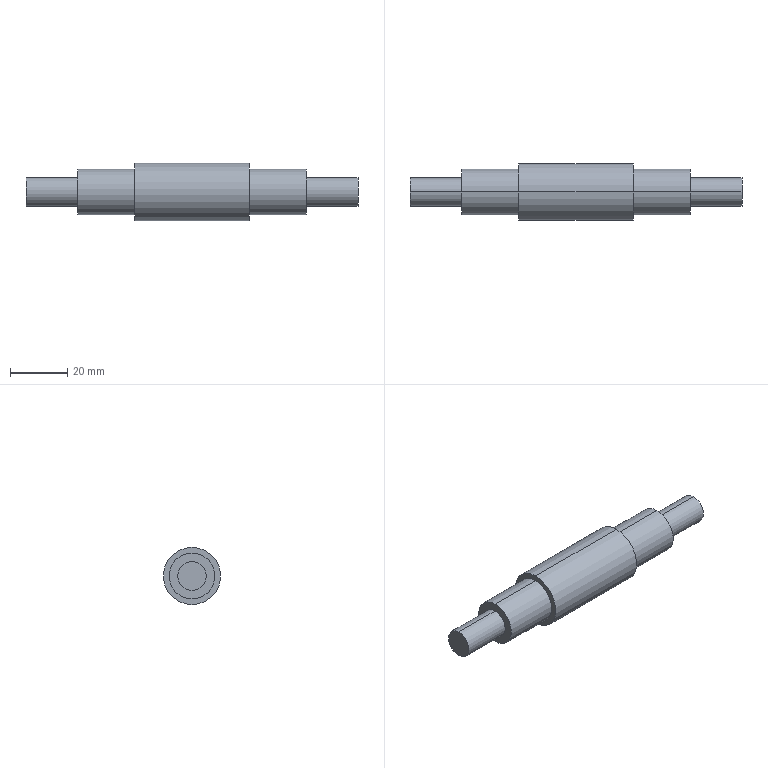Part | SolidWorks | features BaseBody 1 | 1 solid | 16 faces | box 116 x 20 x 20 mm | volume 23436 mm3 | cylinder 10 | plane 6 | commonest cylinder face diameters 10 x4 16 x4 20 x2
STEP:
#1=CARTESIAN_POINT('',(78.,0.,-5.));
#2=VERTEX_POINT('',#1);
#3=CARTESIAN_POINT('',(78.,0.,5.));
#4=VERTEX_POINT('',#3);
#5=CARTESIAN_POINT('',(78.,0.,0.));
#6=DIRECTION('',(1.,0.,0.));
#7=DIRECTION('',(0.,0.,-1.));
#8=AXIS2_PLACEMENT_3D('',#5,#6,#7);
#9=CIRCLE('',#8,5.);
#10=EDGE_CURVE('',#2,#4,#9,.T.);
#11=ORIENTED_EDGE('',*,*,#10,.F.);
#12=CARTESIAN_POINT('',(60.,0.,-5.));
#13=VERTEX_POINT('',#12);
#14=CARTESIAN_POINT('',(78.,0.,-5.));
#15=DIRECTION('',(-1.,0.,0.));
#16=VECTOR('',#15,1000.);
#17=LINE('',#14,#16);
#18=EDGE_CURVE('',#2,#13,#17,.T.);
#19=ORIENTED_EDGE('',*,*,#18,.T.);
#20=CARTESIAN_POINT('',(60.,0.,5.));
#21=VERTEX_POINT('',#20);
#22=CARTESIAN_POINT('',(60.,0.,0.));
#23=DIRECTION('',(1.,0.,0.));
#24=DIRECTION('',(0.,0.,-1.));
#25=AXIS2_PLACEMENT_3D('',#22,#23,#24);
#26=CIRCLE('',#25,5.);
#27=EDGE_CURVE('',#13,#21,#26,.T.);
#28=ORIENTED_EDGE('',*,*,#27,.T.);
#29=CARTESIAN_POINT('',(78.,0.,5.));
#30=DIRECTION('',(-1.,0.,0.));
#31=VECTOR('',#30,1000.);
#32=LINE('',#29,#31);
#33=EDGE_CURVE('',#4,#21,#32,.T.);
#34=ORIENTED_EDGE('',*,*,#33,.F.);
#35=EDGE_LOOP('',(#11,#19,#28,#34));
#36=FACE_OUTER_BOUND('',#35,.T.);
#37=CARTESIAN_POINT('',(78.,0.,0.));
#38=DIRECTION('',(-1.,0.,0.));
#39=DIRECTION('',(0.,0.,1.));
#40=AXIS2_PLACEMENT_3D('',#37,#38,#39);
#41=CYLINDRICAL_SURFACE('',#40,5.);
#42=ADVANCED_FACE('',(#36),#41,.T.);
#43=CARTESIAN_POINT('',(-38.,0.,5.));
#44=VERTEX_POINT('',#43);
#45=CARTESIAN_POINT('',(-38.,0.,-5.));
#46=VERTEX_POINT('',#45);
#47=CARTESIAN_POINT('',(-38.,0.,0.));
#48=DIRECTION('',(-1.,0.,0.));
#49=DIRECTION('',(0.,0.,1.));
#50=AXIS2_PLACEMENT_3D('',#47,#48,#49);
#51=CIRCLE('',#50,5.);
#52=EDGE_CURVE('',#44,#46,#51,.T.);
#53=ORIENTED_EDGE('',*,*,#52,.F.);
#54=CARTESIAN_POINT('',(-20.,0.,5.));
#55=VERTEX_POINT('',#54);
#56=CARTESIAN_POINT('',(-38.,0.,5.));
#57=DIRECTION('',(1.,0.,0.));
#58=VECTOR('',#57,1000.);
#59=LINE('',#56,#58);
#60=EDGE_CURVE('',#44,#55,#59,.T.);
#61=ORIENTED_EDGE('',*,*,#60,.T.);
#62=CARTESIAN_POINT('',(-20.,0.,-5.));
#63=VERTEX_POINT('',#62);
#64=CARTESIAN_POINT('',(-20.,0.,0.));
#65=DIRECTION('',(-1.,0.,0.));
#66=DIRECTION('',(0.,0.,1.));
#67=AXIS2_PLACEMENT_3D('',#64,#65,#66);
#68=CIRCLE('',#67,5.);
#69=EDGE_CURVE('',#55,#63,#68,.T.);
#70=ORIENTED_EDGE('',*,*,#69,.T.);
#71=CARTESIAN_POINT('',(-38.,0.,-5.));
#72=DIRECTION('',(1.,0.,0.));
#73=VECTOR('',#72,1000.);
#74=LINE('',#71,#73);
#75=EDGE_CURVE('',#46,#63,#74,.T.);
#76=ORIENTED_EDGE('',*,*,#75,.F.);
#77=EDGE_LOOP('',(#53,#61,#70,#76));
#78=FACE_OUTER_BOUND('',#77,.T.);
#79=CARTESIAN_POINT('',(-38.,0.,0.));
#80=DIRECTION('',(1.,0.,0.));
#81=DIRECTION('',(0.,0.,-1.));
#82=AXIS2_PLACEMENT_3D('',#79,#80,#81);
#83=CYLINDRICAL_SURFACE('',#82,5.);
#84=ADVANCED_FACE('',(#78),#83,.T.);
#85=CARTESIAN_POINT('',(-20.,0.,8.));
#86=VERTEX_POINT('',#85);
#87=CARTESIAN_POINT('',(-20.,0.,-8.));
#88=VERTEX_POINT('',#87);
#89=CARTESIAN_POINT('',(-20.,0.,0.));
#90=DIRECTION('',(-1.,0.,0.));
#91=DIRECTION('',(0.,0.,1.));
#92=AXIS2_PLACEMENT_3D('',#89,#90,#91);
#93=CIRCLE('',#92,8.);
#94=EDGE_CURVE('',#86,#88,#93,.T.);
#95=ORIENTED_EDGE('',*,*,#94,.F.);
#96=CARTESIAN_POINT('',(0.,0.,8.));
#97=VERTEX_POINT('',#96);
#98=CARTESIAN_POINT('',(-20.,0.,8.));
#99=DIRECTION('',(1.,0.,0.));
#100=VECTOR('',#99,1000.);
#101=LINE('',#98,#100);
#102=EDGE_CURVE('',#86,#97,#101,.T.);
#103=ORIENTED_EDGE('',*,*,#102,.T.);
#104=CARTESIAN_POINT('',(0.,0.,-8.));
#105=VERTEX_POINT('',#104);
#106=CARTESIAN_POINT('',(0.,0.,0.));
#107=DIRECTION('',(-1.,0.,0.));
#108=DIRECTION('',(0.,0.,1.));
#109=AXIS2_PLACEMENT_3D('',#106,#107,#108);
#110=CIRCLE('',#109,8.);
#111=EDGE_CURVE('',#97,#105,#110,.T.);
#112=ORIENTED_EDGE('',*,*,#111,.T.);
#113=CARTESIAN_POINT('',(-20.,0.,-8.));
#114=DIRECTION('',(1.,0.,0.));
#115=VECTOR('',#114,1000.);
#116=LINE('',#113,#115);
#117=EDGE_CURVE('',#88,#105,#116,.T.);
#118=ORIENTED_EDGE('',*,*,#117,.F.);
#119=EDGE_LOOP('',(#95,#103,#112,#118));
#120=FACE_OUTER_BOUND('',#119,.T.);
#121=CARTESIAN_POINT('',(-20.,0.,0.));
#122=DIRECTION('',(1.,0.,0.));
#123=DIRECTION('',(0.,0.,-1.));
#124=AXIS2_PLACEMENT_3D('',#121,#122,#123);
#125=CYLINDRICAL_SURFACE('',#124,8.);
#126=ADVANCED_FACE('',(#120),#125,.T.);
#127=CARTESIAN_POINT('',(60.,0.,-8.));
#128=VERTEX_POINT('',#127);
#129=CARTESIAN_POINT('',(60.,0.,8.));
#130=VERTEX_POINT('',#129);
#131=CARTESIAN_POINT('',(60.,0.,0.));
#132=DIRECTION('',(1.,0.,0.));
#133=DIRECTION('',(0.,0.,-1.));
#134=AXIS2_PLACEMENT_3D('',#131,#132,#133);
#135=CIRCLE('',#134,8.);
#136=EDGE_CURVE('',#128,#130,#135,.T.);
#137=ORIENTED_EDGE('',*,*,#136,.F.);
#138=CARTESIAN_POINT('',(40.,0.,-8.));
#139=VERTEX_POINT('',#138);
#140=CARTESIAN_POINT('',(60.,0.,-8.));
#141=DIRECTION('',(-1.,0.,0.));
#142=VECTOR('',#141,1000.);
#143=LINE('',#140,#142);
#144=EDGE_CURVE('',#128,#139,#143,.T.);
#145=ORIENTED_EDGE('',*,*,#144,.T.);
#146=CARTESIAN_POINT('',(40.,0.,8.));
#147=VERTEX_POINT('',#146);
#148=CARTESIAN_POINT('',(40.,0.,0.));
#149=DIRECTION('',(1.,0.,0.));
#150=DIRECTION('',(0.,0.,-1.));
#151=AXIS2_PLACEMENT_3D('',#148,#149,#150);
#152=CIRCLE('',#151,8.);
#153=EDGE_CURVE('',#139,#147,#152,.T.);
#154=ORIENTED_EDGE('',*,*,#153,.T.);
#155=CARTESIAN_POINT('',(60.,0.,8.));
#156=DIRECTION('',(-1.,0.,0.));
#157=VECTOR('',#156,1000.);
#158=LINE('',#155,#157);
#159=EDGE_CURVE('',#130,#147,#158,.T.);
#160=ORIENTED_EDGE('',*,*,#159,.F.);
#161=EDGE_LOOP('',(#137,#145,#154,#160));
#162=FACE_OUTER_BOUND('',#161,.T.);
#163=CARTESIAN_POINT('',(60.,0.,0.));
#164=DIRECTION('',(-1.,0.,0.));
#165=DIRECTION('',(0.,0.,1.));
#166=AXIS2_PLACEMENT_3D('',#163,#164,#165);
#167=CYLINDRICAL_SURFACE('',#166,8.);
#168=ADVANCED_FACE('',(#162),#167,.T.);
#169=CARTESIAN_POINT('',(40.,0.,-10.));
#170=VERTEX_POINT('',#169);
#171=CARTESIAN_POINT('',(40.,0.,10.));
#172=VERTEX_POINT('',#171);
#173=CARTESIAN_POINT('',(40.,0.,0.));
#174=DIRECTION('',(1.,0.,0.));
#175=DIRECTION('',(0.,0.,-1.));
#176=AXIS2_PLACEMENT_3D('',#173,#174,#175);
#177=CIRCLE('',#176,10.);
#178=EDGE_CURVE('',#170,#172,#177,.T.);
#179=ORIENTED_EDGE('',*,*,#178,.F.);
#180=CARTESIAN_POINT('',(0.,0.,-10.));
#181=VERTEX_POINT('',#180);
#182=CARTESIAN_POINT('',(40.,0.,-10.));
#183=DIRECTION('',(-1.,0.,0.));
#184=VECTOR('',#183,1000.);
#185=LINE('',#182,#184);
#186=EDGE_CURVE('',#170,#181,#185,.T.);
#187=ORIENTED_EDGE('',*,*,#186,.T.);
#188=CARTESIAN_POINT('',(0.,0.,10.));
#189=VERTEX_POINT('',#188);
#190=CARTESIAN_POINT('',(0.,0.,0.));
#191=DIRECTION('',(1.,0.,0.));
#192=DIRECTION('',(0.,0.,-1.));
#193=AXIS2_PLACEMENT_3D('',#190,#191,#192);
#194=CIRCLE('',#193,10.);
#195=EDGE_CURVE('',#181,#189,#194,.T.);
#196=ORIENTED_EDGE('',*,*,#195,.T.);
#197=CARTESIAN_POINT('',(40.,0.,10.));
#198=DIRECTION('',(-1.,0.,0.));
#199=VECTOR('',#198,1000.);
#200=LINE('',#197,#199);
#201=EDGE_CURVE('',#172,#189,#200,.T.);
#202=ORIENTED_EDGE('',*,*,#201,.F.);
#203=EDGE_LOOP('',(#179,#187,#196,#202));
#204=FACE_OUTER_BOUND('',#203,.T.);
#205=CARTESIAN_POINT('',(40.,0.,0.));
#206=DIRECTION('',(-1.,0.,0.));
#207=DIRECTION('',(0.,0.,1.));
#208=AXIS2_PLACEMENT_3D('',#205,#206,#207);
#209=CYLINDRICAL_SURFACE('',#208,10.);
#210=ADVANCED_FACE('',(#204),#209,.T.);
#211=ORIENTED_EDGE('',*,*,#186,.F.);
#212=CARTESIAN_POINT('',(40.,0.,0.));
#213=DIRECTION('',(1.,0.,0.));
#214=DIRECTION('',(0.,0.,-1.));
#215=AXIS2_PLACEMENT_3D('',#212,#213,#214);
#216=CIRCLE('',#215,10.);
#217=EDGE_CURVE('',#172,#170,#216,.T.);
#218=ORIENTED_EDGE('',*,*,#217,.F.);
#219=ORIENTED_EDGE('',*,*,#201,.T.);
#220=CARTESIAN_POINT('',(0.,0.,0.));
#221=DIRECTION('',(1.,0.,0.));
#222=DIRECTION('',(0.,0.,-1.));
#223=AXIS2_PLACEMENT_3D('',#220,#221,#222);
#224=CIRCLE('',#223,10.);
#225=EDGE_CURVE('',#189,#181,#224,.T.);
#226=ORIENTED_EDGE('',*,*,#225,.T.);
#227=EDGE_LOOP('',(#211,#218,#219,#226));
#228=FACE_OUTER_BOUND('',#227,.T.);
#229=CARTESIAN_POINT('',(40.,0.,0.));
#230=DIRECTION('',(-1.,0.,0.));
#231=DIRECTION('',(0.,0.,1.));
#232=AXIS2_PLACEMENT_3D('',#229,#230,#231);
#233=CYLINDRICAL_SURFACE('',#232,10.);
#234=ADVANCED_FACE('',(#228),#233,.T.);
#235=CARTESIAN_POINT('',(40.,0.,0.));
#236=DIRECTION('',(1.,0.,0.));
#237=DIRECTION('',(0.,0.,-1.));
#238=AXIS2_PLACEMENT_3D('',#235,#236,#237);
#239=CIRCLE('',#238,8.);
#240=EDGE_CURVE('',#147,#139,#239,.T.);
#241=ORIENTED_EDGE('',*,*,#240,.F.);
#242=ORIENTED_EDGE('',*,*,#153,.F.);
#243=EDGE_LOOP('',(#241,#242));
#244=FACE_BOUND('',#243,.T.);
#245=ORIENTED_EDGE('',*,*,#217,.T.);
#246=ORIENTED_EDGE('',*,*,#178,.T.);
#247=EDGE_LOOP('',(#245,#246));
#248=FACE_OUTER_BOUND('',#247,.T.);
#249=CARTESIAN_POINT('',(40.,0.,0.));
#250=DIRECTION('',(1.,0.,0.));
#251=DIRECTION('',(0.,0.,-1.));
#252=AXIS2_PLACEMENT_3D('',#249,#250,#251);
#253=PLANE('',#252);
#254=ADVANCED_FACE('',(#244,#248),#253,.T.);
#255=CARTESIAN_POINT('',(0.,0.,0.));
#256=DIRECTION('',(-1.,0.,0.));
#257=DIRECTION('',(0.,0.,1.));
#258=AXIS2_PLACEMENT_3D('',#255,#256,#257);
#259=CIRCLE('',#258,8.);
#260=EDGE_CURVE('',#105,#97,#259,.T.);
#261=ORIENTED_EDGE('',*,*,#260,.F.);
#262=ORIENTED_EDGE('',*,*,#111,.F.);
#263=EDGE_LOOP('',(#261,#262));
#264=FACE_BOUND('',#263,.T.);
#265=ORIENTED_EDGE('',*,*,#225,.F.);
#266=ORIENTED_EDGE('',*,*,#195,.F.);
#267=EDGE_LOOP('',(#265,#266));
#268=FACE_OUTER_BOUND('',#267,.T.);
#269=CARTESIAN_POINT('',(0.,0.,0.));
#270=DIRECTION('',(1.,0.,0.));
#271=DIRECTION('',(0.,0.,-1.));
#272=AXIS2_PLACEMENT_3D('',#269,#270,#271);
#273=PLANE('',#272);
#274=ADVANCED_FACE('',(#264,#268),#273,.F.);
#275=ORIENTED_EDGE('',*,*,#144,.F.);
#276=CARTESIAN_POINT('',(60.,0.,0.));
#277=DIRECTION('',(1.,0.,0.));
#278=DIRECTION('',(0.,0.,-1.));
#279=AXIS2_PLACEMENT_3D('',#276,#277,#278);
#280=CIRCLE('',#279,8.);
#281=EDGE_CURVE('',#130,#128,#280,.T.);
#282=ORIENTED_EDGE('',*,*,#281,.F.);
#283=ORIENTED_EDGE('',*,*,#159,.T.);
#284=ORIENTED_EDGE('',*,*,#240,.T.);
#285=EDGE_LOOP('',(#275,#282,#283,#284));
#286=FACE_OUTER_BOUND('',#285,.T.);
#287=CARTESIAN_POINT('',(60.,0.,0.));
#288=DIRECTION('',(-1.,0.,0.));
#289=DIRECTION('',(0.,0.,1.));
#290=AXIS2_PLACEMENT_3D('',#287,#288,#289);
#291=CYLINDRICAL_SURFACE('',#290,8.);
#292=ADVANCED_FACE('',(#286),#291,.T.);
#293=CARTESIAN_POINT('',(60.,0.,0.));
#294=DIRECTION('',(1.,0.,0.));
#295=DIRECTION('',(0.,0.,-1.));
#296=AXIS2_PLACEMENT_3D('',#293,#294,#295);
#297=CIRCLE('',#296,5.);
#298=EDGE_CURVE('',#21,#13,#297,.T.);
#299=ORIENTED_EDGE('',*,*,#298,.F.);
#300=ORIENTED_EDGE('',*,*,#27,.F.);
#301=EDGE_LOOP('',(#299,#300));
#302=FACE_BOUND('',#301,.T.);
#303=ORIENTED_EDGE('',*,*,#281,.T.);
#304=ORIENTED_EDGE('',*,*,#136,.T.);
#305=EDGE_LOOP('',(#303,#304));
#306=FACE_OUTER_BOUND('',#305,.T.);
#307=CARTESIAN_POINT('',(60.,0.,0.));
#308=DIRECTION('',(1.,0.,0.));
#309=DIRECTION('',(0.,0.,-1.));
#310=AXIS2_PLACEMENT_3D('',#307,#308,#309);
#311=PLANE('',#310);
#312=ADVANCED_FACE('',(#302,#306),#311,.T.);
#313=ORIENTED_EDGE('',*,*,#102,.F.);
#314=CARTESIAN_POINT('',(-20.,0.,0.));
#315=DIRECTION('',(-1.,0.,0.));
#316=DIRECTION('',(0.,0.,1.));
#317=AXIS2_PLACEMENT_3D('',#314,#315,#316);
#318=CIRCLE('',#317,8.);
#319=EDGE_CURVE('',#88,#86,#318,.T.);
#320=ORIENTED_EDGE('',*,*,#319,.F.);
#321=ORIENTED_EDGE('',*,*,#117,.T.);
#322=ORIENTED_EDGE('',*,*,#260,.T.);
#323=EDGE_LOOP('',(#313,#320,#321,#322));
#324=FACE_OUTER_BOUND('',#323,.T.);
#325=CARTESIAN_POINT('',(-20.,0.,0.));
#326=DIRECTION('',(1.,0.,0.));
#327=DIRECTION('',(0.,0.,-1.));
#328=AXIS2_PLACEMENT_3D('',#325,#326,#327);
#329=CYLINDRICAL_SURFACE('',#328,8.);
#330=ADVANCED_FACE('',(#324),#329,.T.);
#331=CARTESIAN_POINT('',(-20.,0.,0.));
#332=DIRECTION('',(-1.,0.,0.));
#333=DIRECTION('',(0.,0.,1.));
#334=AXIS2_PLACEMENT_3D('',#331,#332,#333);
#335=CIRCLE('',#334,5.);
#336=EDGE_CURVE('',#63,#55,#335,.T.);
#337=ORIENTED_EDGE('',*,*,#336,.F.);
#338=ORIENTED_EDGE('',*,*,#69,.F.);
#339=EDGE_LOOP('',(#337,#338));
#340=FACE_BOUND('',#339,.T.);
#341=ORIENTED_EDGE('',*,*,#319,.T.);
#342=ORIENTED_EDGE('',*,*,#94,.T.);
#343=EDGE_LOOP('',(#341,#342));
#344=FACE_OUTER_BOUND('',#343,.T.);
#345=CARTESIAN_POINT('',(-20.,0.,0.));
#346=DIRECTION('',(-1.,0.,0.));
#347=DIRECTION('',(0.,0.,1.));
#348=AXIS2_PLACEMENT_3D('',#345,#346,#347);
#349=PLANE('',#348);
#350=ADVANCED_FACE('',(#340,#344),#349,.T.);
#351=ORIENTED_EDGE('',*,*,#60,.F.);
#352=CARTESIAN_POINT('',(-38.,0.,0.));
#353=DIRECTION('',(-1.,0.,0.));
#354=DIRECTION('',(0.,0.,1.));
#355=AXIS2_PLACEMENT_3D('',#352,#353,#354);
#356=CIRCLE('',#355,5.);
#357=EDGE_CURVE('',#46,#44,#356,.T.);
#358=ORIENTED_EDGE('',*,*,#357,.F.);
#359=ORIENTED_EDGE('',*,*,#75,.T.);
#360=ORIENTED_EDGE('',*,*,#336,.T.);
#361=EDGE_LOOP('',(#351,#358,#359,#360));
#362=FACE_OUTER_BOUND('',#361,.T.);
#363=CARTESIAN_POINT('',(-38.,0.,0.));
#364=DIRECTION('',(1.,0.,0.));
#365=DIRECTION('',(0.,0.,-1.));
#366=AXIS2_PLACEMENT_3D('',#363,#364,#365);
#367=CYLINDRICAL_SURFACE('',#366,5.);
#368=ADVANCED_FACE('',(#362),#367,.T.);
#369=ORIENTED_EDGE('',*,*,#357,.T.);
#370=ORIENTED_EDGE('',*,*,#52,.T.);
#371=EDGE_LOOP('',(#369,#370));
#372=FACE_OUTER_BOUND('',#371,.T.);
#373=CARTESIAN_POINT('',(-38.,0.,0.));
#374=DIRECTION('',(-1.,0.,0.));
#375=DIRECTION('',(0.,0.,1.));
#376=AXIS2_PLACEMENT_3D('',#373,#374,#375);
#377=PLANE('',#376);
#378=ADVANCED_FACE('',(#372),#377,.T.);
#379=ORIENTED_EDGE('',*,*,#18,.F.);
#380=CARTESIAN_POINT('',(78.,0.,0.));
#381=DIRECTION('',(1.,0.,0.));
#382=DIRECTION('',(0.,0.,-1.));
#383=AXIS2_PLACEMENT_3D('',#380,#381,#382);
#384=CIRCLE('',#383,5.);
#385=EDGE_CURVE('',#4,#2,#384,.T.);
#386=ORIENTED_EDGE('',*,*,#385,.F.);
#387=ORIENTED_EDGE('',*,*,#33,.T.);
#388=ORIENTED_EDGE('',*,*,#298,.T.);
#389=EDGE_LOOP('',(#379,#386,#387,#388));
#390=FACE_OUTER_BOUND('',#389,.T.);
#391=CARTESIAN_POINT('',(78.,0.,0.));
#392=DIRECTION('',(-1.,0.,0.));
#393=DIRECTION('',(0.,0.,1.));
#394=AXIS2_PLACEMENT_3D('',#391,#392,#393);
#395=CYLINDRICAL_SURFACE('',#394,5.);
#396=ADVANCED_FACE('',(#390),#395,.T.);
#397=ORIENTED_EDGE('',*,*,#385,.T.);
#398=ORIENTED_EDGE('',*,*,#10,.T.);
#399=EDGE_LOOP('',(#397,#398));
#400=FACE_OUTER_BOUND('',#399,.T.);
#401=CARTESIAN_POINT('',(78.,0.,0.));
#402=DIRECTION('',(1.,0.,0.));
#403=DIRECTION('',(0.,0.,-1.));
#404=AXIS2_PLACEMENT_3D('',#401,#402,#403);
#405=PLANE('',#404);
#406=ADVANCED_FACE('',(#400),#405,.T.);
#407=CLOSED_SHELL('',(#42,#84,#126,#168,#210,#234,#254,#274,#292,#312,#330,#350,#368,#378,#396,#406));
#408=MANIFOLD_SOLID_BREP('',#407);
#409=CARTESIAN_POINT('',(0.,0.,0.));
#410=DIRECTION('',(0.,0.,1.));
#411=DIRECTION('',(1.,0.,0.));
#412=AXIS2_PLACEMENT_3D('',#409,#410,#411);
#413=(LENGTH_UNIT()NAMED_UNIT(*)SI_UNIT(.MILLI.,.METRE.));
#414=UNCERTAINTY_MEASURE_WITH_UNIT(LENGTH_MEASURE(0.00001),#413,'','');
#415=(NAMED_UNIT(*)PLANE_ANGLE_UNIT()SI_UNIT($,.RADIAN.));
#416=(NAMED_UNIT(*)SI_UNIT($,.STERADIAN.)SOLID_ANGLE_UNIT());
#417=(GEOMETRIC_REPRESENTATION_CONTEXT(3)GLOBAL_UNCERTAINTY_ASSIGNED_CONTEXT((#414))GLOBAL_UNIT_ASSIGNED_CONTEXT((#413,#415,#416))REPRESENTATION_CONTEXT('',''));
#418=ADVANCED_BREP_SHAPE_REPRESENTATION('',(#408,#412),#417);